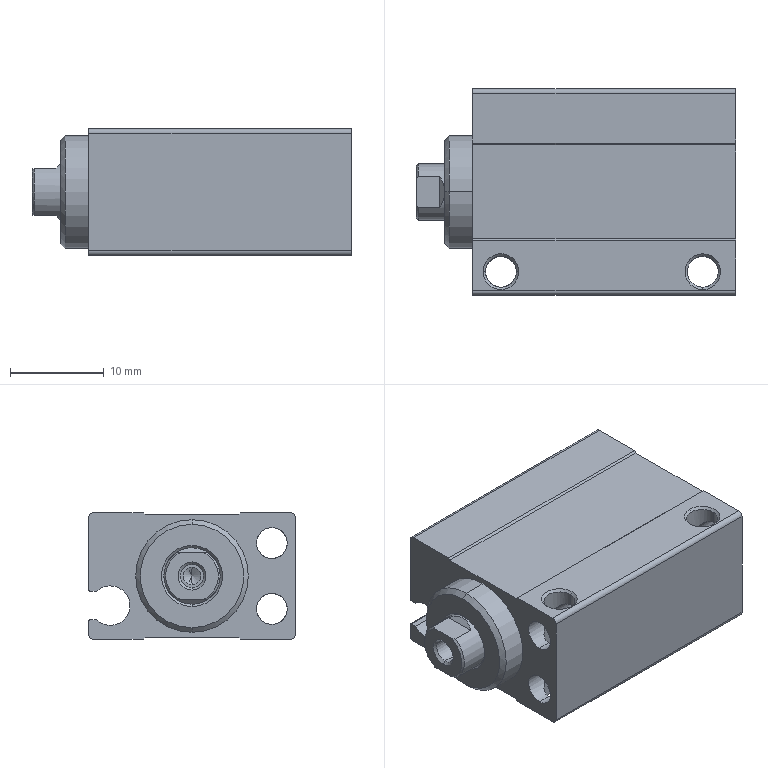Part | STEP file | Compact free-mount cylinder MU10x10S | 2 solids | 144 faces | box 34 x 22 x 13.5 mm | volume 6493 mm3 | cylinder 67 | plane 39 | cone 30 | spline 8 | commonest cylinder face diameters 3.3 x24 1 x8 10 x8 2.459 x6 6 x4 12 x4